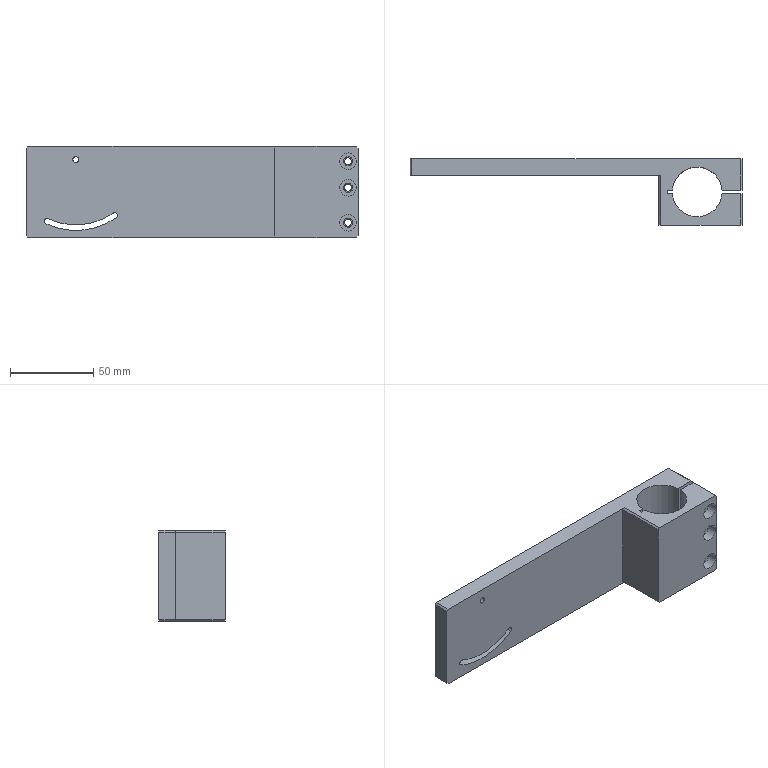CAM job | NX | 3+2 milling, drilling | part box 200 x 40 x 55 mm | stock box 205 x 45 x 60 mm
Tools:
number,name,description,diameter,corner_radius,flute_length,length,flutes
3,D3,平底铣刀-粗,3.0,0.0,20.0,75.0,2
4,D4,平底铣刀-粗,4.0,0.0,25.0,75.0,2
9,D10,平底铣刀-粗,10.0,0.0,35.0,75.0,2
10,D10-J,平底铣刀-精,10.0,0.0,35.0,75.0,2
1,D80R0.8飞刀,圆鼻刀-粗,80.0,0.8,50.0,75.0,2
1,D80R0.8飞刀-J,圆鼻刀-精,80.0,0.8,50.0,75.0,2
2,D6倒角刀,倒角刀,6.0,0.0,3.0,25.0,2
22,M5X0.8,丝锥,4.2,0.0,35.0,50.0,2
17,ZT3.5,钻头,3.5,0.0,35.0,50.0,2
14,ZT4.2,钻头,4.2,0.0,35.0,50.0,2
18,ZT5.5,钻头,5.5,0.0,35.0,50.0,2
Operations:
program,operation,operation_type,tool,method,geometry_group,spindle_rpm,surface_speed,feed_per_tooth,feed_cut,feed_plunge,cut_length_mm,path_length_mm,cut_time_min,machine_time_min
B,底壁铣飞面一刀开粗_COPY,VolumeBased25DMillingOperation,D80R0.8飞刀,分层开粗-切深K-步距G,W-B,5000.0,1256.637,0.3,3000.0,100.0,2773.746,5405.966,0.9246,1.188
B,底壁铣飞面一刀精光_COPY,VolumeBased25DMillingOperation,D80R0.8飞刀-J,侧刃精光-切深K-步距G,W-B,5000.0,1256.637,0.1,1000.0,100.0,307.998,343.998,0.308,0.3116
B,底壁铣分层开粗-中_COPY,VolumeBased25DMillingOperation,D10,分层开粗-切深K-步距G,W-B,8000.0,251.327,0.375,6000.0,100.0,75574.863,83953.703,12.596,13.434
B,打点-深0.8_2,Operation,D6倒角刀,NONE,W-B,8000.0,150.796,0.0312,500.0,90.0,7.2,291.002,0.0144,0.0428
B,三段孔-G83钻孔,Operation,ZT5.5,NONE,W-B,3000.0,39.584,0.0333,200.0,90.0,70.957,220.969,0.3548,0.3698
B,底壁铣螺旋开粗-小_COPY,VolumeBased25DMillingOperation,D4,分层开粗-切深K-步距G,W-B,8000.0,100.528,0.125,2000.0,100.0,1142.87,1328.075,0.5714,0.59
B,底壁铣螺旋精光-小_COPY,VolumeBased25DMillingOperation,D4,螺旋精光-切深K-步距G,W-B,8000.0,100.528,0.05,800.0,100.0,260.451,432.213,0.3256,0.3427
B,钻倒角_2,Operation,D6倒角刀,METHOD,W-B,8000.0,150.796,0.0312,500.0,0.0,5.05,110.1,0.0101,0.0206
B,铣倒角_2,PlanarMilling,D6倒角刀,METHOD,W-B,8000.0,150.796,0.05,800.0,100.0,110.471,273.6,0.1381,0.1544
B,平面去毛刺6X45L_COPY,SurfaceContour,D6倒角刀,爬面_倒角-切深0-步距G,W-B,6500.0,122.519,0.1154,1500.0,100.0,817.66,1383.396,0.5451,0.6017
B,底壁铣精光底面-中_COPY,VolumeBased25DMillingOperation,D10-J,精光步距切深关,W-B,6000.0,188.496,0.125,1500.0,100.0,2144.411,2231.011,1.43,1.438
B,底壁铣精光侧面-中-选底面_COPY,VolumeBased25DMillingOperation,D10-J,侧刃精光-切深K-步距G,W-B,6000.0,188.496,0.0833,1000.0,100.0,149.971,364.553,0.15,0.1714
A,顶面,FaceMilling,D80R0.8飞刀,侧刃精光-切深K-步距G,W-A,5000.0,1256.637,0.1,1000.0,100.0,294.0,330.0,0.294,0.2976
A,外形粗_2,VolumeBased25DMillingOperation,D10,METHOD,W-A,8000.0,251.327,0.3125,5000.0,80.0,28065.987,28144.787,5.613,5.621
A,打点-深0.8,Operation,D6倒角刀,NONE,W-A,8000.0,150.796,0.0312,500.0,90.0,7.2,258.461,0.0144,0.0395
A,通孔-3-4,Operation,ZT3.5,NONE,W-A,3000.0,32.987,0.0333,200.0,90.0,14.052,68.103,0.0703,0.0757
A,通孔-M5螺纹底孔,Operation,ZT4.2,NONE,W-A,3000.0,39.584,0.0583,350.0,90.0,81.785,242.626,0.2337,0.2498
A,通腰槽粗_1,VolumeBased25DMillingOperation,D3,METHOD,W-A,8000.0,75.398,0.05,800.0,100.0,6462.195,6511.195,8.078,8.083
A,腰槽精_1,VolumeBased25DMillingOperation,D3,METHOD,W-A,8000.0,75.398,0.0187,300.0,100.0,310.99,490.541,1.037,1.055
A,仅选体,SurfaceContour,D6倒角刀,METHOD,W-A,8000.0,150.796,0.1875,3000.0,100.0,623.658,760.575,0.2079,0.2216
A,钻倒角_1,Operation,D6倒角刀,METHOD,W-A,8000.0,150.796,0.0312,500.0,0.0,5.05,50.1,0.0101,0.0146
A,铣倒角_1,PlanarMilling,D6倒角刀,METHOD,W-A,8000.0,150.796,0.0312,500.0,100.0,54.061,214.167,0.1081,0.1241
A,通孔-攻牙M5,Operation,M5X0.8,METHOD,W-A,500.0,6.597,0.0008,0.8,90.0,70.5,220.055,88.125,88.14
A,外形半精_2,VolumeBased25DMillingOperation,D10-J,METHOD,W-A,8000.0,251.327,0.0625,1000.0,100.0,1632.093,1915.322,1.632,1.66